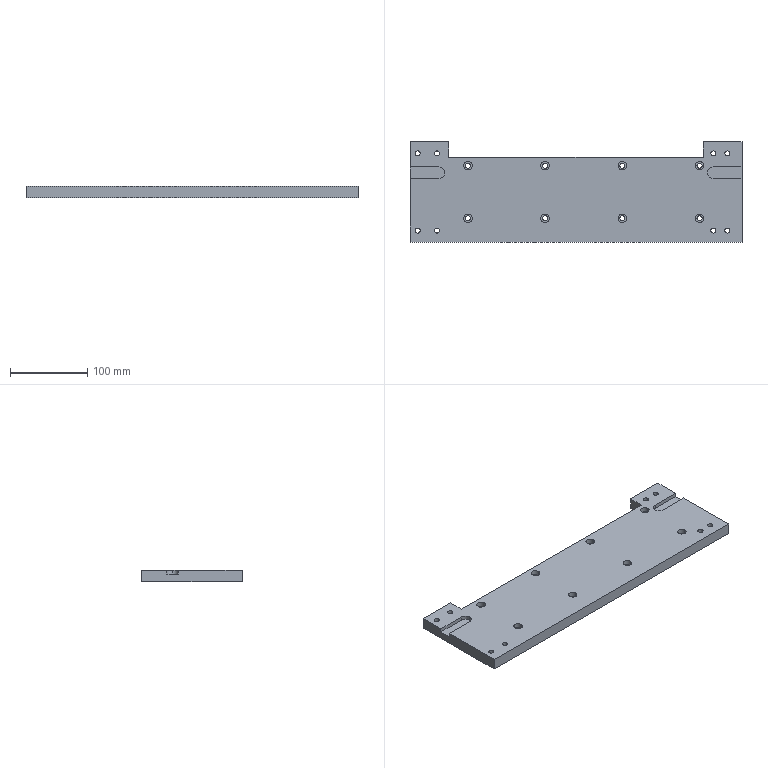Part | SolidWorks | features HoleWzd 2, Cut 1, Extrusion 1, ICE 1 | 1 solid | 99 faces | box 430 x 130 x 15 mm | volume 718358 mm3 | cylinder 67 | plane 32 | commonest cylinder face diameters 6.6 x32 11 x32 15 x3